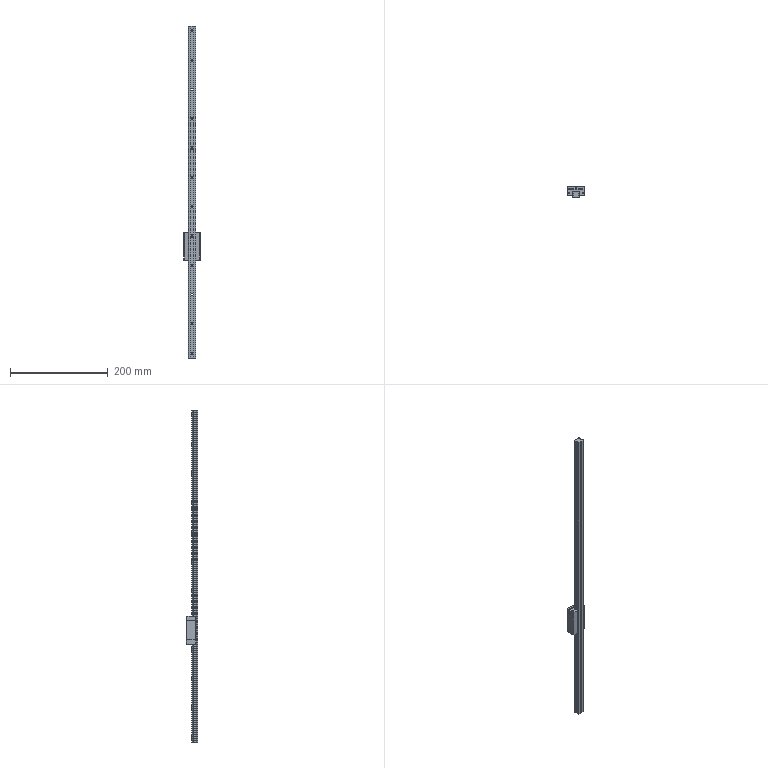Part | SolidWorks | 2 solids | 508 faces | box 34 x 24 x 680 mm | volume 137302 mm3 | plane 309 | cylinder 131 | spline 68 | commonest cylinder face diameters 4.5 x24 8 x24 1.6 x16 0.6 x15 2.1 x12 4 x12